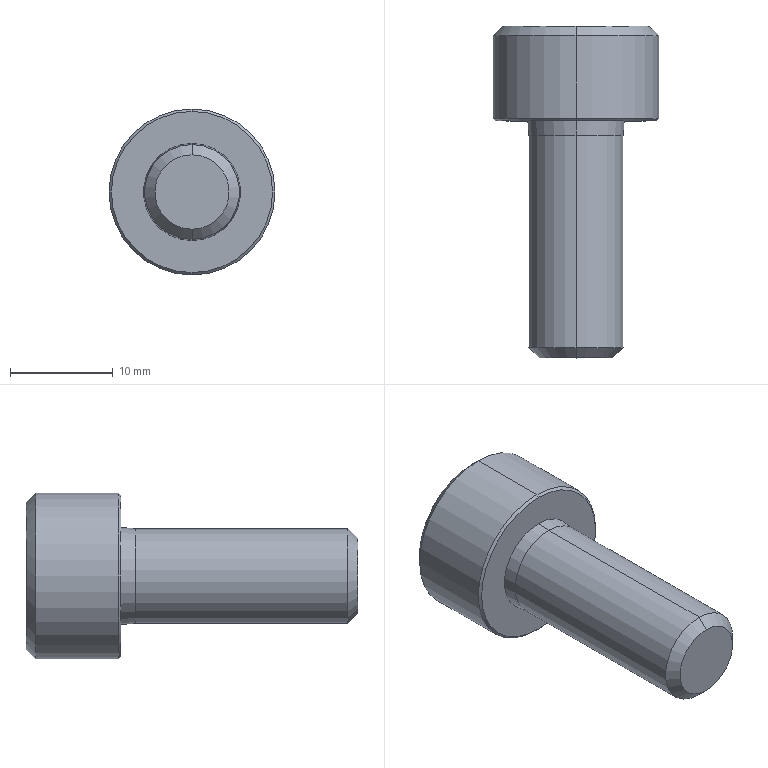Part | SolidWorks | features BaseBody 1 | 1 solid | 36 faces | box 16.154 x 32.308 x 16.154 mm | volume 3185 mm3 | cone 17 | plane 15 | cylinder 4 | commonest cylinder face diameters 9.231 x2 16.154 x2
STEP:
#1=CARTESIAN_POINT('',(207.247,296.414,227.692));
#2=VERTEX_POINT('',#1);
#3=CARTESIAN_POINT('',(207.247,296.414,218.462));
#4=VERTEX_POINT('',#3);
#5=CARTESIAN_POINT('',(207.247,296.414,223.077));
#6=DIRECTION('',(0.,1.,0.));
#7=DIRECTION('',(0.,0.,1.));
#8=AXIS2_PLACEMENT_3D('',#5,#6,#7);
#9=CIRCLE('',#8,4.615);
#10=EDGE_CURVE('',#2,#4,#9,.T.);
#11=ORIENTED_EDGE('',*,*,#10,.T.);
#12=CARTESIAN_POINT('',(207.247,317.115,218.462));
#13=VERTEX_POINT('',#12);
#14=CARTESIAN_POINT('',(207.247,295.423,218.462));
#15=DIRECTION('',(0.,1.,0.));
#16=VECTOR('',#15,1000.);
#17=LINE('',#14,#16);
#18=EDGE_CURVE('',#4,#13,#17,.T.);
#19=ORIENTED_EDGE('',*,*,#18,.T.);
#20=CARTESIAN_POINT('',(207.247,317.115,227.692));
#21=VERTEX_POINT('',#20);
#22=CARTESIAN_POINT('',(207.247,317.115,223.077));
#23=DIRECTION('',(0.,-1.,0.));
#24=DIRECTION('',(0.,0.,1.));
#25=AXIS2_PLACEMENT_3D('',#22,#23,#24);
#26=CIRCLE('',#25,4.615);
#27=EDGE_CURVE('',#13,#21,#26,.T.);
#28=ORIENTED_EDGE('',*,*,#27,.T.);
#29=CARTESIAN_POINT('',(207.247,295.423,227.692));
#30=DIRECTION('',(0.,1.,0.));
#31=VECTOR('',#30,1000.);
#32=LINE('',#29,#31);
#33=EDGE_CURVE('',#2,#21,#32,.T.);
#34=ORIENTED_EDGE('',*,*,#33,.F.);
#35=EDGE_LOOP('',(#11,#19,#28,#34));
#36=FACE_OUTER_BOUND('',#35,.T.);
#37=CARTESIAN_POINT('',(207.247,295.423,223.077));
#38=DIRECTION('',(0.,1.,0.));
#39=DIRECTION('',(0.,0.,1.));
#40=AXIS2_PLACEMENT_3D('',#37,#38,#39);
#41=CYLINDRICAL_SURFACE('',#40,4.615);
#42=ADVANCED_FACE('',(#36),#41,.T.);
#43=CARTESIAN_POINT('',(207.247,295.423,226.701));
#44=VERTEX_POINT('',#43);
#45=CARTESIAN_POINT('',(207.247,295.423,219.453));
#46=VERTEX_POINT('',#45);
#47=CARTESIAN_POINT('',(207.247,295.423,223.077));
#48=DIRECTION('',(0.,1.,0.));
#49=DIRECTION('',(0.,0.,1.));
#50=AXIS2_PLACEMENT_3D('',#47,#48,#49);
#51=CIRCLE('',#50,3.624);
#52=EDGE_CURVE('',#44,#46,#51,.T.);
#53=ORIENTED_EDGE('',*,*,#52,.T.);
#54=CARTESIAN_POINT('',(207.247,296.414,218.462));
#55=DIRECTION('',(0.,0.7071,-0.7071));
#56=VECTOR('',#55,1000.);
#57=LINE('',#54,#56);
#58=EDGE_CURVE('',#46,#4,#57,.T.);
#59=ORIENTED_EDGE('',*,*,#58,.T.);
#60=ORIENTED_EDGE('',*,*,#10,.F.);
#61=CARTESIAN_POINT('',(207.247,296.414,227.692));
#62=DIRECTION('',(0.,0.7071,0.7071));
#63=VECTOR('',#62,1000.);
#64=LINE('',#61,#63);
#65=EDGE_CURVE('',#44,#2,#64,.T.);
#66=ORIENTED_EDGE('',*,*,#65,.F.);
#67=EDGE_LOOP('',(#53,#59,#60,#66));
#68=FACE_OUTER_BOUND('',#67,.T.);
#69=CARTESIAN_POINT('',(207.247,296.414,223.077));
#70=DIRECTION('',(0.,1.,0.));
#71=DIRECTION('',(0.,0.,1.));
#72=AXIS2_PLACEMENT_3D('',#69,#70,#71);
#73=CONICAL_SURFACE('',#72,4.615,0.7854);
#74=ADVANCED_FACE('',(#68),#73,.T.);
#75=ORIENTED_EDGE('',*,*,#27,.F.);
#76=CARTESIAN_POINT('',(207.247,318.5,218.346));
#77=VERTEX_POINT('',#76);
#78=CARTESIAN_POINT('',(207.247,318.5,218.346));
#79=DIRECTION('',(0.,0.9965,-0.08305));
#80=VECTOR('',#79,1000.);
#81=LINE('',#78,#80);
#82=EDGE_CURVE('',#13,#77,#81,.T.);
#83=ORIENTED_EDGE('',*,*,#82,.T.);
#84=CARTESIAN_POINT('',(207.247,318.5,227.808));
#85=VERTEX_POINT('',#84);
#86=CARTESIAN_POINT('',(207.247,318.5,223.077));
#87=DIRECTION('',(0.,-1.,0.));
#88=DIRECTION('',(0.,0.,1.));
#89=AXIS2_PLACEMENT_3D('',#86,#87,#88);
#90=CIRCLE('',#89,4.731);
#91=EDGE_CURVE('',#77,#85,#90,.T.);
#92=ORIENTED_EDGE('',*,*,#91,.T.);
#93=CARTESIAN_POINT('',(207.247,318.5,227.808));
#94=DIRECTION('',(0.,0.9965,0.08305));
#95=VECTOR('',#94,1000.);
#96=LINE('',#93,#95);
#97=EDGE_CURVE('',#21,#85,#96,.T.);
#98=ORIENTED_EDGE('',*,*,#97,.F.);
#99=EDGE_LOOP('',(#75,#83,#92,#98));
#100=FACE_OUTER_BOUND('',#99,.T.);
#101=CARTESIAN_POINT('',(207.247,318.5,223.077));
#102=DIRECTION('',(0.,1.,0.));
#103=DIRECTION('',(0.,0.,1.));
#104=AXIS2_PLACEMENT_3D('',#101,#102,#103);
#105=CONICAL_SURFACE('',#104,4.731,0.08314);
#106=ADVANCED_FACE('',(#100),#105,.T.);
#107=CARTESIAN_POINT('',(207.247,318.5,230.923));
#108=VERTEX_POINT('',#107);
#109=CARTESIAN_POINT('',(207.247,318.5,215.231));
#110=VERTEX_POINT('',#109);
#111=CARTESIAN_POINT('',(207.247,318.5,223.077));
#112=DIRECTION('',(0.,1.,0.));
#113=DIRECTION('',(0.,0.,1.));
#114=AXIS2_PLACEMENT_3D('',#111,#112,#113);
#115=CIRCLE('',#114,7.846);
#116=EDGE_CURVE('',#108,#110,#115,.T.);
#117=ORIENTED_EDGE('',*,*,#116,.T.);
#118=CARTESIAN_POINT('',(207.247,318.731,215.));
#119=VERTEX_POINT('',#118);
#120=CARTESIAN_POINT('',(207.247,318.731,215.));
#121=DIRECTION('',(0.,0.7071,-0.7071));
#122=VECTOR('',#121,1000.);
#123=LINE('',#120,#122);
#124=EDGE_CURVE('',#110,#119,#123,.T.);
#125=ORIENTED_EDGE('',*,*,#124,.T.);
#126=CARTESIAN_POINT('',(207.247,318.731,231.154));
#127=VERTEX_POINT('',#126);
#128=CARTESIAN_POINT('',(207.247,318.731,223.077));
#129=DIRECTION('',(0.,-1.,0.));
#130=DIRECTION('',(0.,0.,-1.));
#131=AXIS2_PLACEMENT_3D('',#128,#129,#130);
#132=CIRCLE('',#131,8.077);
#133=EDGE_CURVE('',#119,#127,#132,.T.);
#134=ORIENTED_EDGE('',*,*,#133,.T.);
#135=CARTESIAN_POINT('',(207.247,318.731,231.154));
#136=DIRECTION('',(0.,0.7071,0.7071));
#137=VECTOR('',#136,1000.);
#138=LINE('',#135,#137);
#139=EDGE_CURVE('',#108,#127,#138,.T.);
#140=ORIENTED_EDGE('',*,*,#139,.F.);
#141=EDGE_LOOP('',(#117,#125,#134,#140));
#142=FACE_OUTER_BOUND('',#141,.T.);
#143=CARTESIAN_POINT('',(207.247,318.731,223.077));
#144=DIRECTION('',(0.,1.,0.));
#145=DIRECTION('',(0.,0.,1.));
#146=AXIS2_PLACEMENT_3D('',#143,#144,#145);
#147=CONICAL_SURFACE('',#146,8.077,0.7854);
#148=ADVANCED_FACE('',(#142),#147,.T.);
#149=ORIENTED_EDGE('',*,*,#133,.F.);
#150=CARTESIAN_POINT('',(207.247,326.808,215.));
#151=VERTEX_POINT('',#150);
#152=CARTESIAN_POINT('',(207.247,295.423,215.));
#153=DIRECTION('',(0.,1.,0.));
#154=VECTOR('',#153,1000.);
#155=LINE('',#152,#154);
#156=EDGE_CURVE('',#119,#151,#155,.T.);
#157=ORIENTED_EDGE('',*,*,#156,.T.);
#158=CARTESIAN_POINT('',(207.247,326.808,231.154));
#159=VERTEX_POINT('',#158);
#160=CARTESIAN_POINT('',(207.247,326.808,223.077));
#161=DIRECTION('',(0.,-1.,0.));
#162=DIRECTION('',(0.,0.,1.));
#163=AXIS2_PLACEMENT_3D('',#160,#161,#162);
#164=CIRCLE('',#163,8.077);
#165=EDGE_CURVE('',#151,#159,#164,.T.);
#166=ORIENTED_EDGE('',*,*,#165,.T.);
#167=CARTESIAN_POINT('',(207.247,295.423,231.154));
#168=DIRECTION('',(0.,1.,0.));
#169=VECTOR('',#168,1000.);
#170=LINE('',#167,#169);
#171=EDGE_CURVE('',#127,#159,#170,.T.);
#172=ORIENTED_EDGE('',*,*,#171,.F.);
#173=EDGE_LOOP('',(#149,#157,#166,#172));
#174=FACE_OUTER_BOUND('',#173,.T.);
#175=CARTESIAN_POINT('',(207.247,295.423,223.077));
#176=DIRECTION('',(0.,1.,0.));
#177=DIRECTION('',(0.,0.,1.));
#178=AXIS2_PLACEMENT_3D('',#175,#176,#177);
#179=CYLINDRICAL_SURFACE('',#178,8.077);
#180=ADVANCED_FACE('',(#174),#179,.T.);
#181=CARTESIAN_POINT('',(207.247,327.731,215.923));
#182=VERTEX_POINT('',#181);
#183=CARTESIAN_POINT('',(207.247,327.731,230.231));
#184=VERTEX_POINT('',#183);
#185=CARTESIAN_POINT('',(207.247,327.731,223.077));
#186=DIRECTION('',(0.,-1.,0.));
#187=DIRECTION('',(0.,0.,-1.));
#188=AXIS2_PLACEMENT_3D('',#185,#186,#187);
#189=CIRCLE('',#188,7.154);
#190=EDGE_CURVE('',#182,#184,#189,.T.);
#191=ORIENTED_EDGE('',*,*,#190,.T.);
#192=CARTESIAN_POINT('',(207.247,326.808,231.154));
#193=DIRECTION('',(0.,-0.7071,0.7071));
#194=VECTOR('',#193,1000.);
#195=LINE('',#192,#194);
#196=EDGE_CURVE('',#184,#159,#195,.T.);
#197=ORIENTED_EDGE('',*,*,#196,.T.);
#198=ORIENTED_EDGE('',*,*,#165,.F.);
#199=CARTESIAN_POINT('',(207.247,326.808,215.));
#200=DIRECTION('',(0.,-0.7071,-0.7071));
#201=VECTOR('',#200,1000.);
#202=LINE('',#199,#201);
#203=EDGE_CURVE('',#182,#151,#202,.T.);
#204=ORIENTED_EDGE('',*,*,#203,.F.);
#205=EDGE_LOOP('',(#191,#197,#198,#204));
#206=FACE_OUTER_BOUND('',#205,.T.);
#207=CARTESIAN_POINT('',(207.247,326.808,223.077));
#208=DIRECTION('',(0.,-1.,0.));
#209=DIRECTION('',(0.,0.,-1.));
#210=AXIS2_PLACEMENT_3D('',#207,#208,#209);
#211=CONICAL_SURFACE('',#210,8.077,0.7854);
#212=ADVANCED_FACE('',(#206),#211,.T.);
#213=CARTESIAN_POINT('',(207.247,327.195,226.538));
#214=VERTEX_POINT('',#213);
#215=CARTESIAN_POINT('',(209.245,327.731,226.538));
#216=VERTEX_POINT('',#215);
#217=CARTESIAN_POINT('',(207.247,327.195,226.538));
#218=CARTESIAN_POINT('',(207.594,327.195,226.538));
#219=CARTESIAN_POINT('',(207.936,327.248,226.538));
#220=CARTESIAN_POINT('',(208.61,327.44,226.538));
#221=CARTESIAN_POINT('',(208.932,327.574,226.538));
#222=CARTESIAN_POINT('',(209.245,327.731,226.538));
#223=B_SPLINE_CURVE_WITH_KNOTS('',3,(#217,#218,#219,#220,#221,#222),.UNSPECIFIED.,.F.,.F.,(4,2,4),(0.002072,0.0031,0.004129),.UNSPECIFIED.);
#224=EDGE_CURVE('',#214,#216,#223,.T.);
#225=ORIENTED_EDGE('',*,*,#224,.F.);
#226=CARTESIAN_POINT('',(207.247,327.731,227.074));
#227=VERTEX_POINT('',#226);
#228=CARTESIAN_POINT('',(207.247,327.731,227.074));
#229=DIRECTION('',(0.,0.7071,0.7071));
#230=VECTOR('',#229,1000.);
#231=LINE('',#228,#230);
#232=EDGE_CURVE('',#214,#227,#231,.T.);
#233=ORIENTED_EDGE('',*,*,#232,.T.);
#234=CARTESIAN_POINT('',(207.247,327.731,223.077));
#235=DIRECTION('',(0.,1.,0.));
#236=DIRECTION('',(0.,0.,1.));
#237=AXIS2_PLACEMENT_3D('',#234,#235,#236);
#238=CIRCLE('',#237,3.997);
#239=EDGE_CURVE('',#227,#216,#238,.T.);
#240=ORIENTED_EDGE('',*,*,#239,.T.);
#241=EDGE_LOOP('',(#225,#233,#240));
#242=FACE_OUTER_BOUND('',#241,.T.);
#243=CARTESIAN_POINT('',(207.247,327.731,223.077));
#244=DIRECTION('',(0.,1.,0.));
#245=DIRECTION('',(0.,0.,1.));
#246=AXIS2_PLACEMENT_3D('',#243,#244,#245);
#247=CONICAL_SURFACE('',#246,3.997,0.7854);
#248=ADVANCED_FACE('',(#242),#247,.F.);
#249=CARTESIAN_POINT('',(207.247,321.117,223.077));
#250=VERTEX_POINT('',#249);
#251=CARTESIAN_POINT('',(207.247,323.115,226.538));
#252=VERTEX_POINT('',#251);
#253=CARTESIAN_POINT('',(207.247,323.115,226.538));
#254=DIRECTION('',(0.,0.5,0.866));
#255=VECTOR('',#254,1000.);
#256=LINE('',#253,#255);
#257=EDGE_CURVE('',#250,#252,#256,.T.);
#258=ORIENTED_EDGE('',*,*,#257,.F.);
#259=CARTESIAN_POINT('',(207.247,323.115,219.615));
#260=VERTEX_POINT('',#259);
#261=CARTESIAN_POINT('',(207.247,323.115,219.615));
#262=DIRECTION('',(0.,0.5,-0.866));
#263=VECTOR('',#262,1000.);
#264=LINE('',#261,#263);
#265=EDGE_CURVE('',#250,#260,#264,.T.);
#266=ORIENTED_EDGE('',*,*,#265,.T.);
#267=CARTESIAN_POINT('',(204.249,323.115,221.346));
#268=VERTEX_POINT('',#267);
#269=CARTESIAN_POINT('',(207.247,323.115,223.077));
#270=DIRECTION('',(0.,-1.,0.));
#271=DIRECTION('',(0.,0.,1.));
#272=AXIS2_PLACEMENT_3D('',#269,#270,#271);
#273=CIRCLE('',#272,3.462);
#274=EDGE_CURVE('',#268,#260,#273,.T.);
#275=ORIENTED_EDGE('',*,*,#274,.F.);
#276=CARTESIAN_POINT('',(204.249,323.115,224.808));
#277=VERTEX_POINT('',#276);
#278=CARTESIAN_POINT('',(207.247,323.115,223.077));
#279=DIRECTION('',(0.,-1.,0.));
#280=DIRECTION('',(0.,0.,1.));
#281=AXIS2_PLACEMENT_3D('',#278,#279,#280);
#282=CIRCLE('',#281,3.462);
#283=EDGE_CURVE('',#277,#268,#282,.T.);
#284=ORIENTED_EDGE('',*,*,#283,.F.);
#285=CARTESIAN_POINT('',(207.247,323.115,223.077));
#286=DIRECTION('',(0.,-1.,0.));
#287=DIRECTION('',(0.,0.,1.));
#288=AXIS2_PLACEMENT_3D('',#285,#286,#287);
#289=CIRCLE('',#288,3.462);
#290=EDGE_CURVE('',#252,#277,#289,.T.);
#291=ORIENTED_EDGE('',*,*,#290,.F.);
#292=EDGE_LOOP('',(#258,#266,#275,#284,#291));
#293=FACE_OUTER_BOUND('',#292,.T.);
#294=CARTESIAN_POINT('',(207.247,323.115,223.077));
#295=DIRECTION('',(0.,1.,0.));
#296=DIRECTION('',(0.,0.,1.));
#297=AXIS2_PLACEMENT_3D('',#294,#295,#296);
#298=CONICAL_SURFACE('',#297,3.462,1.047);
#299=ADVANCED_FACE('',(#293),#298,.F.);
#300=ORIENTED_EDGE('',*,*,#18,.F.);
#301=CARTESIAN_POINT('',(207.247,296.414,223.077));
#302=DIRECTION('',(0.,1.,0.));
#303=DIRECTION('',(0.,0.,1.));
#304=AXIS2_PLACEMENT_3D('',#301,#302,#303);
#305=CIRCLE('',#304,4.615);
#306=EDGE_CURVE('',#4,#2,#305,.T.);
#307=ORIENTED_EDGE('',*,*,#306,.T.);
#308=ORIENTED_EDGE('',*,*,#33,.T.);
#309=CARTESIAN_POINT('',(207.247,317.115,223.077));
#310=DIRECTION('',(0.,-1.,0.));
#311=DIRECTION('',(0.,0.,1.));
#312=AXIS2_PLACEMENT_3D('',#309,#310,#311);
#313=CIRCLE('',#312,4.615);
#314=EDGE_CURVE('',#21,#13,#313,.T.);
#315=ORIENTED_EDGE('',*,*,#314,.T.);
#316=EDGE_LOOP('',(#300,#307,#308,#315));
#317=FACE_OUTER_BOUND('',#316,.T.);
#318=CARTESIAN_POINT('',(207.247,295.423,223.077));
#319=DIRECTION('',(0.,1.,0.));
#320=DIRECTION('',(0.,0.,1.));
#321=AXIS2_PLACEMENT_3D('',#318,#319,#320);
#322=CYLINDRICAL_SURFACE('',#321,4.615);
#323=ADVANCED_FACE('',(#317),#322,.T.);
#324=ORIENTED_EDGE('',*,*,#58,.F.);
#325=CARTESIAN_POINT('',(207.247,295.423,223.077));
#326=DIRECTION('',(0.,1.,0.));
#327=DIRECTION('',(0.,0.,1.));
#328=AXIS2_PLACEMENT_3D('',#325,#326,#327);
#329=CIRCLE('',#328,3.624);
#330=EDGE_CURVE('',#46,#44,#329,.T.);
#331=ORIENTED_EDGE('',*,*,#330,.T.);
#332=ORIENTED_EDGE('',*,*,#65,.T.);
#333=ORIENTED_EDGE('',*,*,#306,.F.);
#334=EDGE_LOOP('',(#324,#331,#332,#333));
#335=FACE_OUTER_BOUND('',#334,.T.);
#336=CARTESIAN_POINT('',(207.247,296.414,223.077));
#337=DIRECTION('',(0.,1.,0.));
#338=DIRECTION('',(0.,0.,1.));
#339=AXIS2_PLACEMENT_3D('',#336,#337,#338);
#340=CONICAL_SURFACE('',#339,4.615,0.7854);
#341=ADVANCED_FACE('',(#335),#340,.T.);
#342=ORIENTED_EDGE('',*,*,#82,.F.);
#343=ORIENTED_EDGE('',*,*,#314,.F.);
#344=ORIENTED_EDGE('',*,*,#97,.T.);
#345=CARTESIAN_POINT('',(207.247,318.5,223.077));
#346=DIRECTION('',(0.,-1.,0.));
#347=DIRECTION('',(0.,0.,1.));
#348=AXIS2_PLACEMENT_3D('',#345,#346,#347);
#349=CIRCLE('',#348,4.731);
#350=EDGE_CURVE('',#85,#77,#349,.T.);
#351=ORIENTED_EDGE('',*,*,#350,.T.);
#352=EDGE_LOOP('',(#342,#343,#344,#351));
#353=FACE_OUTER_BOUND('',#352,.T.);
#354=CARTESIAN_POINT('',(207.247,318.5,223.077));
#355=DIRECTION('',(0.,1.,0.));
#356=DIRECTION('',(0.,0.,1.));
#357=AXIS2_PLACEMENT_3D('',#354,#355,#356);
#358=CONICAL_SURFACE('',#357,4.731,0.08314);
#359=ADVANCED_FACE('',(#353),#358,.T.);
#360=ORIENTED_EDGE('',*,*,#52,.F.);
#361=ORIENTED_EDGE('',*,*,#330,.F.);
#362=EDGE_LOOP('',(#360,#361));
#363=FACE_OUTER_BOUND('',#362,.T.);
#364=CARTESIAN_POINT('',(207.247,295.423,219.453));
#365=DIRECTION('',(0.,1.,0.));
#366=DIRECTION('',(0.,0.,1.));
#367=AXIS2_PLACEMENT_3D('',#364,#365,#366);
#368=PLANE('',#367);
#369=ADVANCED_FACE('',(#363),#368,.F.);
#370=ORIENTED_EDGE('',*,*,#350,.F.);
#371=ORIENTED_EDGE('',*,*,#91,.F.);
#372=EDGE_LOOP('',(#370,#371));
#373=FACE_BOUND('',#372,.T.);
#374=ORIENTED_EDGE('',*,*,#116,.F.);
#375=CARTESIAN_POINT('',(207.247,318.5,223.077));
#376=DIRECTION('',(0.,1.,0.));
#377=DIRECTION('',(0.,0.,1.));
#378=AXIS2_PLACEMENT_3D('',#375,#376,#377);
#379=CIRCLE('',#378,7.846);
#380=EDGE_CURVE('',#110,#108,#379,.T.);
#381=ORIENTED_EDGE('',*,*,#380,.F.);
#382=EDGE_LOOP('',(#374,#381));
#383=FACE_OUTER_BOUND('',#382,.T.);
#384=CARTESIAN_POINT('',(207.247,318.5,215.231));
#385=DIRECTION('',(0.,1.,0.));
#386=DIRECTION('',(0.,0.,1.));
#387=AXIS2_PLACEMENT_3D('',#384,#385,#386);
#388=PLANE('',#387);
#389=ADVANCED_FACE('',(#373,#383),#388,.F.);
#390=ORIENTED_EDGE('',*,*,#124,.F.);
#391=ORIENTED_EDGE('',*,*,#380,.T.);
#392=ORIENTED_EDGE('',*,*,#139,.T.);
#393=CARTESIAN_POINT('',(207.247,318.731,223.077));
#394=DIRECTION('',(0.,-1.,0.));
#395=DIRECTION('',(0.,0.,-1.));
#396=AXIS2_PLACEMENT_3D('',#393,#394,#395);
#397=CIRCLE('',#396,8.077);
#398=EDGE_CURVE('',#127,#119,#397,.T.);
#399=ORIENTED_EDGE('',*,*,#398,.T.);
#400=EDGE_LOOP('',(#390,#391,#392,#399));
#401=FACE_OUTER_BOUND('',#400,.T.);
#402=CARTESIAN_POINT('',(207.247,318.731,223.077));
#403=DIRECTION('',(0.,1.,0.));
#404=DIRECTION('',(0.,0.,1.));
#405=AXIS2_PLACEMENT_3D('',#402,#403,#404);
#406=CONICAL_SURFACE('',#405,8.077,0.7854);
#407=ADVANCED_FACE('',(#401),#406,.T.);
#408=ORIENTED_EDGE('',*,*,#156,.F.);
#409=ORIENTED_EDGE('',*,*,#398,.F.);
#410=ORIENTED_EDGE('',*,*,#171,.T.);
#411=CARTESIAN_POINT('',(207.247,326.808,223.077));
#412=DIRECTION('',(0.,-1.,0.));
#413=DIRECTION('',(0.,0.,1.));
#414=AXIS2_PLACEMENT_3D('',#411,#412,#413);
#415=CIRCLE('',#414,8.077);
#416=EDGE_CURVE('',#159,#151,#415,.T.);
#417=ORIENTED_EDGE('',*,*,#416,.T.);
#418=EDGE_LOOP('',(#408,#409,#410,#417));
#419=FACE_OUTER_BOUND('',#418,.T.);
#420=CARTESIAN_POINT('',(207.247,295.423,223.077));
#421=DIRECTION('',(0.,1.,0.));
#422=DIRECTION('',(0.,0.,1.));
#423=AXIS2_PLACEMENT_3D('',#420,#421,#422);
#424=CYLINDRICAL_SURFACE('',#423,8.077);
#425=ADVANCED_FACE('',(#419),#424,.T.);
#426=ORIENTED_EDGE('',*,*,#196,.F.);
#427=CARTESIAN_POINT('',(207.247,327.731,223.077));
#428=DIRECTION('',(0.,-1.,0.));
#429=DIRECTION('',(0.,0.,-1.));
#430=AXIS2_PLACEMENT_3D('',#427,#428,#429);
#431=CIRCLE('',#430,7.154);
#432=EDGE_CURVE('',#184,#182,#431,.T.);
#433=ORIENTED_EDGE('',*,*,#432,.T.);
#434=ORIENTED_EDGE('',*,*,#203,.T.);
#435=ORIENTED_EDGE('',*,*,#416,.F.);
#436=EDGE_LOOP('',(#426,#433,#434,#435));
#437=FACE_OUTER_BOUND('',#436,.T.);
#438=CARTESIAN_POINT('',(207.247,326.808,223.077));
#439=DIRECTION('',(0.,-1.,0.));
#440=DIRECTION('',(0.,0.,-1.));
#441=AXIS2_PLACEMENT_3D('',#438,#439,#440);
#442=CONICAL_SURFACE('',#441,8.077,0.7854);
#443=ADVANCED_FACE('',(#437),#442,.T.);
#444=CARTESIAN_POINT('',(211.244,327.731,223.077));
#445=VERTEX_POINT('',#444);
#446=CARTESIAN_POINT('',(207.247,327.731,223.077));
#447=DIRECTION('',(0.,1.,0.));
#448=DIRECTION('',(0.,0.,1.));
#449=AXIS2_PLACEMENT_3D('',#446,#447,#448);
#450=CIRCLE('',#449,3.997);
#451=EDGE_CURVE('',#216,#445,#450,.T.);
#452=ORIENTED_EDGE('',*,*,#451,.F.);
#453=ORIENTED_EDGE('',*,*,#239,.F.);
#454=CARTESIAN_POINT('',(205.248,327.731,226.538));
#455=VERTEX_POINT('',#454);
#456=CARTESIAN_POINT('',(207.247,327.731,223.077));
#457=DIRECTION('',(0.,1.,0.));
#458=DIRECTION('',(0.,0.,1.));
#459=AXIS2_PLACEMENT_3D('',#456,#457,#458);
#460=CIRCLE('',#459,3.997);
#461=EDGE_CURVE('',#455,#227,#460,.T.);
#462=ORIENTED_EDGE('',*,*,#461,.F.);
#463=CARTESIAN_POINT('',(203.249,327.731,223.077));
#464=VERTEX_POINT('',#463);
#465=CARTESIAN_POINT('',(207.247,327.731,223.077));
#466=DIRECTION('',(0.,1.,0.));
#467=DIRECTION('',(0.,0.,1.));
#468=AXIS2_PLACEMENT_3D('',#465,#466,#467);
#469=CIRCLE('',#468,3.997);
#470=EDGE_CURVE('',#464,#455,#469,.T.);
#471=ORIENTED_EDGE('',*,*,#470,.F.);
#472=CARTESIAN_POINT('',(205.248,327.731,219.615));
#473=VERTEX_POINT('',#472);
#474=CARTESIAN_POINT('',(207.247,327.731,223.077));
#475=DIRECTION('',(0.,1.,0.));
#476=DIRECTION('',(0.,0.,1.));
#477=AXIS2_PLACEMENT_3D('',#474,#475,#476);
#478=CIRCLE('',#477,3.997);
#479=EDGE_CURVE('',#473,#464,#478,.T.);
#480=ORIENTED_EDGE('',*,*,#479,.F.);
#481=CARTESIAN_POINT('',(209.245,327.731,219.615));
#482=VERTEX_POINT('',#481);
#483=CARTESIAN_POINT('',(207.247,327.731,223.077));
#484=DIRECTION('',(0.,1.,0.));
#485=DIRECTION('',(0.,0.,1.));
#486=AXIS2_PLACEMENT_3D('',#483,#484,#485);
#487=CIRCLE('',#486,3.997);
#488=EDGE_CURVE('',#482,#473,#487,.T.);
#489=ORIENTED_EDGE('',*,*,#488,.F.);
#490=CARTESIAN_POINT('',(207.247,327.731,223.077));
#491=DIRECTION('',(0.,1.,0.));
#492=DIRECTION('',(0.,0.,1.));
#493=AXIS2_PLACEMENT_3D('',#490,#491,#492);
#494=CIRCLE('',#493,3.997);
#495=EDGE_CURVE('',#445,#482,#494,.T.);
#496=ORIENTED_EDGE('',*,*,#495,.F.);
#497=EDGE_LOOP('',(#452,#453,#462,#471,#480,#489,#496));
#498=FACE_BOUND('',#497,.T.);
#499=ORIENTED_EDGE('',*,*,#190,.F.);
#500=ORIENTED_EDGE('',*,*,#432,.F.);
#501=EDGE_LOOP('',(#499,#500));
#502=FACE_OUTER_BOUND('',#501,.T.);
#503=CARTESIAN_POINT('',(207.247,327.731,219.08));
#504=DIRECTION('',(0.,-1.,0.));
#505=DIRECTION('',(0.,0.,-1.));
#506=AXIS2_PLACEMENT_3D('',#503,#504,#505);
#507=PLANE('',#506);
#508=ADVANCED_FACE('',(#498,#502),#507,.F.);
#509=CARTESIAN_POINT('',(211.244,327.731,223.077));
#510=CARTESIAN_POINT('',(211.087,327.575,222.806));
#511=CARTESIAN_POINT('',(210.928,327.442,222.53));
#512=CARTESIAN_POINT('',(210.68,327.3,222.1));
#513=CARTESIAN_POINT('',(210.596,327.262,221.955));
#514=CARTESIAN_POINT('',(210.424,327.21,221.657));
#515=CARTESIAN_POINT('',(210.335,327.196,221.504));
#516=CARTESIAN_POINT('',(210.074,327.195,221.05));
#517=CARTESIAN_POINT('',(209.902,327.247,220.753));
#518=CARTESIAN_POINT('',(209.564,327.439,220.168));
#519=CARTESIAN_POINT('',(209.402,327.574,219.887));
#520=CARTESIAN_POINT('',(209.245,327.731,219.615));
#521=B_SPLINE_CURVE_WITH_KNOTS('',3,(#509,#510,#511,#512,#513,#514,#515,#516,#517,#518,#519,#520),.UNSPECIFIED.,.F.,.F.,(4,2,2,2,2,4),(0.,0.001032,0.001548,0.002064,0.003097,0.004129),.UNSPECIFIED.);
#522=EDGE_CURVE('',#445,#482,#521,.T.);
#523=ORIENTED_EDGE('',*,*,#522,.F.);
#524=ORIENTED_EDGE('',*,*,#495,.T.);
#525=EDGE_LOOP('',(#523,#524));
#526=FACE_OUTER_BOUND('',#525,.T.);
#527=CARTESIAN_POINT('',(207.247,327.731,223.077));
#528=DIRECTION('',(0.,1.,0.));
#529=DIRECTION('',(0.,0.,1.));
#530=AXIS2_PLACEMENT_3D('',#527,#528,#529);
#531=CONICAL_SURFACE('',#530,3.997,0.7854);
#532=ADVANCED_FACE('',(#526),#531,.F.);
#533=CARTESIAN_POINT('',(209.245,327.731,226.538));
#534=CARTESIAN_POINT('',(209.401,327.575,226.268));
#535=CARTESIAN_POINT('',(209.561,327.442,225.991));
#536=CARTESIAN_POINT('',(209.809,327.3,225.562));
#537=CARTESIAN_POINT('',(209.893,327.262,225.416));
#538=CARTESIAN_POINT('',(210.065,327.21,225.118));
#539=CARTESIAN_POINT('',(210.153,327.196,224.965));
#540=CARTESIAN_POINT('',(210.415,327.195,224.512));
#541=CARTESIAN_POINT('',(210.587,327.247,224.215));
#542=CARTESIAN_POINT('',(210.925,327.439,223.629));
#543=CARTESIAN_POINT('',(211.087,327.574,223.349));
#544=CARTESIAN_POINT('',(211.244,327.731,223.077));
#545=B_SPLINE_CURVE_WITH_KNOTS('',3,(#533,#534,#535,#536,#537,#538,#539,#540,#541,#542,#543,#544),.UNSPECIFIED.,.F.,.F.,(4,2,2,2,2,4),(0.,0.001032,0.001548,0.002064,0.003097,0.004129),.UNSPECIFIED.);
#546=EDGE_CURVE('',#216,#445,#545,.T.);
#547=ORIENTED_EDGE('',*,*,#546,.F.);
#548=ORIENTED_EDGE('',*,*,#451,.T.);
#549=EDGE_LOOP('',(#547,#548));
#550=FACE_OUTER_BOUND('',#549,.T.);
#551=CARTESIAN_POINT('',(207.247,327.731,223.077));
#552=DIRECTION('',(0.,1.,0.));
#553=DIRECTION('',(0.,0.,1.));
#554=AXIS2_PLACEMENT_3D('',#551,#552,#553);
#555=CONICAL_SURFACE('',#554,3.997,0.7854);
#556=ADVANCED_FACE('',(#550),#555,.F.);
#557=ORIENTED_EDGE('',*,*,#232,.F.);
#558=CARTESIAN_POINT('',(205.248,327.731,226.538));
#559=CARTESIAN_POINT('',(205.561,327.574,226.538));
#560=CARTESIAN_POINT('',(205.882,327.441,226.538));
#561=CARTESIAN_POINT('',(206.38,327.299,226.538));
#562=CARTESIAN_POINT('',(206.549,327.261,226.538));
#563=CARTESIAN_POINT('',(206.894,327.209,226.538));
#564=CARTESIAN_POINT('',(207.071,327.195,226.538));
#565=CARTESIAN_POINT('',(207.247,327.195,226.538));
#566=B_SPLINE_CURVE_WITH_KNOTS('',3,(#558,#559,#560,#561,#562,#563,#564,#565),.UNSPECIFIED.,.F.,.F.,(4,2,2,4),(0.,0.001036,0.001554,0.002072),.UNSPECIFIED.);
#567=EDGE_CURVE('',#455,#214,#566,.T.);
#568=ORIENTED_EDGE('',*,*,#567,.F.);
#569=ORIENTED_EDGE('',*,*,#461,.T.);
#570=EDGE_LOOP('',(#557,#568,#569));
#571=FACE_OUTER_BOUND('',#570,.T.);
#572=CARTESIAN_POINT('',(207.247,327.731,223.077));
#573=DIRECTION('',(0.,1.,0.));
#574=DIRECTION('',(0.,0.,1.));
#575=AXIS2_PLACEMENT_3D('',#572,#573,#574);
#576=CONICAL_SURFACE('',#575,3.997,0.7854);
#577=ADVANCED_FACE('',(#571),#576,.F.);
#578=CARTESIAN_POINT('',(203.249,327.731,223.077));
#579=CARTESIAN_POINT('',(203.406,327.575,223.347));
#580=CARTESIAN_POINT('',(203.565,327.442,223.624));
#581=CARTESIAN_POINT('',(203.813,327.3,224.054));
#582=CARTESIAN_POINT('',(203.898,327.262,224.199));
#583=CARTESIAN_POINT('',(204.069,327.21,224.497));
#584=CARTESIAN_POINT('',(204.158,327.196,224.65));
#585=CARTESIAN_POINT('',(204.42,327.195,225.104));
#586=CARTESIAN_POINT('',(204.591,327.247,225.401));
#587=CARTESIAN_POINT('',(204.929,327.439,225.986));
#588=CARTESIAN_POINT('',(205.091,327.574,226.266));
#589=CARTESIAN_POINT('',(205.248,327.731,226.538));
#590=B_SPLINE_CURVE_WITH_KNOTS('',3,(#578,#579,#580,#581,#582,#583,#584,#585,#586,#587,#588,#589),.UNSPECIFIED.,.F.,.F.,(4,2,2,2,2,4),(0.,0.001032,0.001548,0.002064,0.003097,0.004129),.UNSPECIFIED.);
#591=EDGE_CURVE('',#464,#455,#590,.T.);
#592=ORIENTED_EDGE('',*,*,#591,.F.);
#593=ORIENTED_EDGE('',*,*,#470,.T.);
#594=EDGE_LOOP('',(#592,#593));
#595=FACE_OUTER_BOUND('',#594,.T.);
#596=CARTESIAN_POINT('',(207.247,327.731,223.077));
#597=DIRECTION('',(0.,1.,0.));
#598=DIRECTION('',(0.,0.,1.));
#599=AXIS2_PLACEMENT_3D('',#596,#597,#598);
#600=CONICAL_SURFACE('',#599,3.997,0.7854);
#601=ADVANCED_FACE('',(#595),#600,.F.);
#602=CARTESIAN_POINT('',(205.248,327.731,219.615));
#603=CARTESIAN_POINT('',(205.092,327.575,219.886));
#604=CARTESIAN_POINT('',(204.932,327.442,220.162));
#605=CARTESIAN_POINT('',(204.684,327.3,220.592));
#606=CARTESIAN_POINT('',(204.6,327.262,220.738));
#607=CARTESIAN_POINT('',(204.428,327.21,221.035));
#608=CARTESIAN_POINT('',(204.34,327.196,221.189));
#609=CARTESIAN_POINT('',(204.078,327.195,221.642));
#610=CARTESIAN_POINT('',(203.906,327.247,221.939));
#611=CARTESIAN_POINT('',(203.568,327.439,222.525));
#612=CARTESIAN_POINT('',(203.407,327.574,222.805));
#613=CARTESIAN_POINT('',(203.249,327.731,223.077));
#614=B_SPLINE_CURVE_WITH_KNOTS('',3,(#602,#603,#604,#605,#606,#607,#608,#609,#610,#611,#612,#613),.UNSPECIFIED.,.F.,.F.,(4,2,2,2,2,4),(0.,0.001032,0.001548,0.002064,0.003097,0.004129),.UNSPECIFIED.);
#615=EDGE_CURVE('',#473,#464,#614,.T.);
#616=ORIENTED_EDGE('',*,*,#615,.F.);
#617=ORIENTED_EDGE('',*,*,#479,.T.);
#618=EDGE_LOOP('',(#616,#617));
#619=FACE_OUTER_BOUND('',#618,.T.);
#620=CARTESIAN_POINT('',(207.247,327.731,223.077));
#621=DIRECTION('',(0.,1.,0.));
#622=DIRECTION('',(0.,0.,1.));
#623=AXIS2_PLACEMENT_3D('',#620,#621,#622);
#624=CONICAL_SURFACE('',#623,3.997,0.7854);
#625=ADVANCED_FACE('',(#619),#624,.F.);
#626=CARTESIAN_POINT('',(209.245,327.731,219.615));
#627=CARTESIAN_POINT('',(208.933,327.575,219.615));
#628=CARTESIAN_POINT('',(208.613,327.442,219.615));
#629=CARTESIAN_POINT('',(208.117,327.3,219.615));
#630=CARTESIAN_POINT('',(207.949,327.262,219.615));
#631=CARTESIAN_POINT('',(207.605,327.21,219.615));
#632=CARTESIAN_POINT('',(207.428,327.196,219.615));
#633=CARTESIAN_POINT('',(206.905,327.195,219.615));
#634=CARTESIAN_POINT('',(206.562,327.247,219.615));
#635=CARTESIAN_POINT('',(205.886,327.439,219.615));
#636=CARTESIAN_POINT('',(205.562,327.574,219.615));
#637=CARTESIAN_POINT('',(205.248,327.731,219.615));
#638=B_SPLINE_CURVE_WITH_KNOTS('',3,(#626,#627,#628,#629,#630,#631,#632,#633,#634,#635,#636,#637),.UNSPECIFIED.,.F.,.F.,(4,2,2,2,2,4),(0.,0.001032,0.001548,0.002064,0.003097,0.004129),.UNSPECIFIED.);
#639=EDGE_CURVE('',#482,#473,#638,.T.);
#640=ORIENTED_EDGE('',*,*,#639,.F.);
#641=ORIENTED_EDGE('',*,*,#488,.T.);
#642=EDGE_LOOP('',(#640,#641));
#643=FACE_OUTER_BOUND('',#642,.T.);
#644=CARTESIAN_POINT('',(207.247,327.731,223.077));
#645=DIRECTION('',(0.,1.,0.));
#646=DIRECTION('',(0.,0.,1.));
#647=AXIS2_PLACEMENT_3D('',#644,#645,#646);
#648=CONICAL_SURFACE('',#647,3.997,0.7854);
#649=ADVANCED_FACE('',(#643),#648,.F.);
#650=CARTESIAN_POINT('',(209.245,323.115,219.615));
#651=VERTEX_POINT('',#650);
#652=CARTESIAN_POINT('',(209.245,323.115,219.615));
#653=DIRECTION('',(0.,1.,0.));
#654=VECTOR('',#653,1000.);
#655=LINE('',#652,#654);
#656=EDGE_CURVE('',#651,#482,#655,.T.);
#657=ORIENTED_EDGE('',*,*,#656,.F.);
#658=CARTESIAN_POINT('',(210.244,323.115,221.346));
#659=VERTEX_POINT('',#658);
#660=CARTESIAN_POINT('',(211.244,323.115,223.077));
#661=DIRECTION('',(-0.5,0.,-0.866));
#662=VECTOR('',#661,1000.);
#663=LINE('',#660,#662);
#664=EDGE_CURVE('',#659,#651,#663,.T.);
#665=ORIENTED_EDGE('',*,*,#664,.F.);
#666=CARTESIAN_POINT('',(211.244,323.115,223.077));
#667=VERTEX_POINT('',#666);
#668=CARTESIAN_POINT('',(211.244,323.115,223.077));
#669=DIRECTION('',(-0.5,0.,-0.866));
#670=VECTOR('',#669,1000.);
#671=LINE('',#668,#670);
#672=EDGE_CURVE('',#667,#659,#671,.T.);
#673=ORIENTED_EDGE('',*,*,#672,.F.);
#674=CARTESIAN_POINT('',(211.244,323.115,223.077));
#675=DIRECTION('',(0.,-1.,0.));
#676=VECTOR('',#675,1000.);
#677=LINE('',#674,#676);
#678=EDGE_CURVE('',#445,#667,#677,.T.);
#679=ORIENTED_EDGE('',*,*,#678,.F.);
#680=ORIENTED_EDGE('',*,*,#522,.T.);
#681=EDGE_LOOP('',(#657,#665,#673,#679,#680));
#682=FACE_OUTER_BOUND('',#681,.T.);
#683=CARTESIAN_POINT('',(211.244,323.115,223.077));
#684=DIRECTION('',(0.866,0.,-0.5));
#685=DIRECTION('',(-0.5,0.,-0.866));
#686=AXIS2_PLACEMENT_3D('',#683,#684,#685);
#687=PLANE('',#686);
#688=ADVANCED_FACE('',(#682),#687,.F.);
#689=ORIENTED_EDGE('',*,*,#678,.T.);
#690=CARTESIAN_POINT('',(210.244,323.115,224.808));
#691=VERTEX_POINT('',#690);
#692=CARTESIAN_POINT('',(209.245,323.115,226.538));
#693=DIRECTION('',(0.5,0.,-0.866));
#694=VECTOR('',#693,1000.);
#695=LINE('',#692,#694);
#696=EDGE_CURVE('',#691,#667,#695,.T.);
#697=ORIENTED_EDGE('',*,*,#696,.F.);
#698=CARTESIAN_POINT('',(209.245,323.115,226.538));
#699=VERTEX_POINT('',#698);
#700=CARTESIAN_POINT('',(209.245,323.115,226.538));
#701=DIRECTION('',(0.5,0.,-0.866));
#702=VECTOR('',#701,1000.);
#703=LINE('',#700,#702);
#704=EDGE_CURVE('',#699,#691,#703,.T.);
#705=ORIENTED_EDGE('',*,*,#704,.F.);
#706=CARTESIAN_POINT('',(209.245,323.115,226.538));
#707=DIRECTION('',(0.,-1.,0.));
#708=VECTOR('',#707,1000.);
#709=LINE('',#706,#708);
#710=EDGE_CURVE('',#216,#699,#709,.T.);
#711=ORIENTED_EDGE('',*,*,#710,.F.);
#712=ORIENTED_EDGE('',*,*,#546,.T.);
#713=EDGE_LOOP('',(#689,#697,#705,#711,#712));
#714=FACE_OUTER_BOUND('',#713,.T.);
#715=CARTESIAN_POINT('',(209.245,323.115,226.538));
#716=DIRECTION('',(0.866,0.,0.5));
#717=DIRECTION('',(0.5,0.,-0.866));
#718=AXIS2_PLACEMENT_3D('',#715,#716,#717);
#719=PLANE('',#718);
#720=ADVANCED_FACE('',(#714),#719,.F.);
#721=ORIENTED_EDGE('',*,*,#710,.T.);
#722=CARTESIAN_POINT('',(205.248,323.115,226.538));
#723=DIRECTION('',(1.,0.,0.));
#724=VECTOR('',#723,1000.);
#725=LINE('',#722,#724);
#726=EDGE_CURVE('',#252,#699,#725,.T.);
#727=ORIENTED_EDGE('',*,*,#726,.F.);
#728=CARTESIAN_POINT('',(205.248,323.115,226.538));
#729=VERTEX_POINT('',#728);
#730=CARTESIAN_POINT('',(205.248,323.115,226.538));
#731=DIRECTION('',(1.,0.,0.));
#732=VECTOR('',#731,1000.);
#733=LINE('',#730,#732);
#734=EDGE_CURVE('',#729,#252,#733,.T.);
#735=ORIENTED_EDGE('',*,*,#734,.F.);
#736=CARTESIAN_POINT('',(205.248,323.115,226.538));
#737=DIRECTION('',(0.,-1.,0.));
#738=VECTOR('',#737,1000.);
#739=LINE('',#736,#738);
#740=EDGE_CURVE('',#455,#729,#739,.T.);
#741=ORIENTED_EDGE('',*,*,#740,.F.);
#742=ORIENTED_EDGE('',*,*,#567,.T.);
#743=ORIENTED_EDGE('',*,*,#224,.T.);
#744=EDGE_LOOP('',(#721,#727,#735,#741,#742,#743));
#745=FACE_OUTER_BOUND('',#744,.T.);
#746=CARTESIAN_POINT('',(205.248,323.115,226.538));
#747=DIRECTION('',(0.,0.,1.));
#748=DIRECTION('',(1.,0.,0.));
#749=AXIS2_PLACEMENT_3D('',#746,#747,#748);
#750=PLANE('',#749);
#751=ADVANCED_FACE('',(#745),#750,.F.);
#752=ORIENTED_EDGE('',*,*,#740,.T.);
#753=CARTESIAN_POINT('',(203.249,323.115,223.077));
#754=DIRECTION('',(0.5,0.,0.866));
#755=VECTOR('',#754,1000.);
#756=LINE('',#753,#755);
#757=EDGE_CURVE('',#277,#729,#756,.T.);
#758=ORIENTED_EDGE('',*,*,#757,.F.);
#759=CARTESIAN_POINT('',(203.249,323.115,223.077));
#760=VERTEX_POINT('',#759);
#761=CARTESIAN_POINT('',(203.249,323.115,223.077));
#762=DIRECTION('',(0.5,0.,0.866));
#763=VECTOR('',#762,1000.);
#764=LINE('',#761,#763);
#765=EDGE_CURVE('',#760,#277,#764,.T.);
#766=ORIENTED_EDGE('',*,*,#765,.F.);
#767=CARTESIAN_POINT('',(203.249,323.115,223.077));
#768=DIRECTION('',(0.,-1.,0.));
#769=VECTOR('',#768,1000.);
#770=LINE('',#767,#769);
#771=EDGE_CURVE('',#464,#760,#770,.T.);
#772=ORIENTED_EDGE('',*,*,#771,.F.);
#773=ORIENTED_EDGE('',*,*,#591,.T.);
#774=EDGE_LOOP('',(#752,#758,#766,#772,#773));
#775=FACE_OUTER_BOUND('',#774,.T.);
#776=CARTESIAN_POINT('',(203.249,323.115,223.077));
#777=DIRECTION('',(-0.866,0.,0.5));
#778=DIRECTION('',(0.5,0.,0.866));
#779=AXIS2_PLACEMENT_3D('',#776,#777,#778);
#780=PLANE('',#779);
#781=ADVANCED_FACE('',(#775),#780,.F.);
#782=ORIENTED_EDGE('',*,*,#771,.T.);
#783=CARTESIAN_POINT('',(205.248,323.115,219.615));
#784=DIRECTION('',(-0.5,0.,0.866));
#785=VECTOR('',#784,1000.);
#786=LINE('',#783,#785);
#787=EDGE_CURVE('',#268,#760,#786,.T.);
#788=ORIENTED_EDGE('',*,*,#787,.F.);
#789=CARTESIAN_POINT('',(205.248,323.115,219.615));
#790=VERTEX_POINT('',#789);
#791=CARTESIAN_POINT('',(205.248,323.115,219.615));
#792=DIRECTION('',(-0.5,0.,0.866));
#793=VECTOR('',#792,1000.);
#794=LINE('',#791,#793);
#795=EDGE_CURVE('',#790,#268,#794,.T.);
#796=ORIENTED_EDGE('',*,*,#795,.F.);
#797=CARTESIAN_POINT('',(205.248,323.115,219.615));
#798=DIRECTION('',(0.,-1.,0.));
#799=VECTOR('',#798,1000.);
#800=LINE('',#797,#799);
#801=EDGE_CURVE('',#473,#790,#800,.T.);
#802=ORIENTED_EDGE('',*,*,#801,.F.);
#803=ORIENTED_EDGE('',*,*,#615,.T.);
#804=EDGE_LOOP('',(#782,#788,#796,#802,#803));
#805=FACE_OUTER_BOUND('',#804,.T.);
#806=CARTESIAN_POINT('',(205.248,323.115,219.615));
#807=DIRECTION('',(-0.866,0.,-0.5));
#808=DIRECTION('',(-0.5,0.,0.866));
#809=AXIS2_PLACEMENT_3D('',#806,#807,#808);
#810=PLANE('',#809);
#811=ADVANCED_FACE('',(#805),#810,.F.);
#812=ORIENTED_EDGE('',*,*,#801,.T.);
#813=CARTESIAN_POINT('',(209.245,323.115,219.615));
#814=DIRECTION('',(-1.,0.,0.));
#815=VECTOR('',#814,1000.);
#816=LINE('',#813,#815);
#817=EDGE_CURVE('',#260,#790,#816,.T.);
#818=ORIENTED_EDGE('',*,*,#817,.F.);
#819=CARTESIAN_POINT('',(209.245,323.115,219.615));
#820=DIRECTION('',(-1.,0.,0.));
#821=VECTOR('',#820,1000.);
#822=LINE('',#819,#821);
#823=EDGE_CURVE('',#651,#260,#822,.T.);
#824=ORIENTED_EDGE('',*,*,#823,.F.);
#825=ORIENTED_EDGE('',*,*,#656,.T.);
#826=ORIENTED_EDGE('',*,*,#639,.T.);
#827=EDGE_LOOP('',(#812,#818,#824,#825,#826));
#828=FACE_OUTER_BOUND('',#827,.T.);
#829=CARTESIAN_POINT('',(209.245,323.115,219.615));
#830=DIRECTION('',(0.,0.,-1.));
#831=DIRECTION('',(-1.,0.,0.));
#832=AXIS2_PLACEMENT_3D('',#829,#830,#831);
#833=PLANE('',#832);
#834=ADVANCED_FACE('',(#828),#833,.F.);
#835=CARTESIAN_POINT('',(207.247,323.115,223.077));
#836=DIRECTION('',(0.,-1.,0.));
#837=DIRECTION('',(0.,0.,1.));
#838=AXIS2_PLACEMENT_3D('',#835,#836,#837);
#839=CIRCLE('',#838,3.462);
#840=EDGE_CURVE('',#260,#659,#839,.T.);
#841=ORIENTED_EDGE('',*,*,#840,.T.);
#842=ORIENTED_EDGE('',*,*,#664,.T.);
#843=ORIENTED_EDGE('',*,*,#823,.T.);
#844=EDGE_LOOP('',(#841,#842,#843));
#845=FACE_OUTER_BOUND('',#844,.T.);
#846=CARTESIAN_POINT('',(207.247,323.115,223.077));
#847=DIRECTION('',(0.,1.,0.));
#848=DIRECTION('',(0.,0.,1.));
#849=AXIS2_PLACEMENT_3D('',#846,#847,#848);
#850=PLANE('',#849);
#851=ADVANCED_FACE('',(#845),#850,.T.);
#852=CARTESIAN_POINT('',(207.247,323.115,223.077));
#853=DIRECTION('',(0.,-1.,0.));
#854=DIRECTION('',(0.,0.,1.));
#855=AXIS2_PLACEMENT_3D('',#852,#853,#854);
#856=CIRCLE('',#855,3.462);
#857=EDGE_CURVE('',#659,#691,#856,.T.);
#858=ORIENTED_EDGE('',*,*,#857,.T.);
#859=ORIENTED_EDGE('',*,*,#696,.T.);
#860=ORIENTED_EDGE('',*,*,#672,.T.);
#861=EDGE_LOOP('',(#858,#859,#860));
#862=FACE_OUTER_BOUND('',#861,.T.);
#863=CARTESIAN_POINT('',(207.247,323.115,223.077));
#864=DIRECTION('',(0.,1.,0.));
#865=DIRECTION('',(0.,0.,1.));
#866=AXIS2_PLACEMENT_3D('',#863,#864,#865);
#867=PLANE('',#866);
#868=ADVANCED_FACE('',(#862),#867,.T.);
#869=CARTESIAN_POINT('',(207.247,323.115,223.077));
#870=DIRECTION('',(0.,-1.,0.));
#871=DIRECTION('',(0.,0.,1.));
#872=AXIS2_PLACEMENT_3D('',#869,#870,#871);
#873=CIRCLE('',#872,3.462);
#874=EDGE_CURVE('',#691,#252,#873,.T.);
#875=ORIENTED_EDGE('',*,*,#874,.T.);
#876=ORIENTED_EDGE('',*,*,#726,.T.);
#877=ORIENTED_EDGE('',*,*,#704,.T.);
#878=EDGE_LOOP('',(#875,#876,#877));
#879=FACE_OUTER_BOUND('',#878,.T.);
#880=CARTESIAN_POINT('',(207.247,323.115,223.077));
#881=DIRECTION('',(0.,1.,0.));
#882=DIRECTION('',(0.,0.,1.));
#883=AXIS2_PLACEMENT_3D('',#880,#881,#882);
#884=PLANE('',#883);
#885=ADVANCED_FACE('',(#879),#884,.T.);
#886=ORIENTED_EDGE('',*,*,#290,.T.);
#887=ORIENTED_EDGE('',*,*,#757,.T.);
#888=ORIENTED_EDGE('',*,*,#734,.T.);
#889=EDGE_LOOP('',(#886,#887,#888));
#890=FACE_OUTER_BOUND('',#889,.T.);
#891=CARTESIAN_POINT('',(207.247,323.115,223.077));
#892=DIRECTION('',(0.,1.,0.));
#893=DIRECTION('',(0.,0.,1.));
#894=AXIS2_PLACEMENT_3D('',#891,#892,#893);
#895=PLANE('',#894);
#896=ADVANCED_FACE('',(#890),#895,.T.);
#897=ORIENTED_EDGE('',*,*,#283,.T.);
#898=ORIENTED_EDGE('',*,*,#787,.T.);
#899=ORIENTED_EDGE('',*,*,#765,.T.);
#900=EDGE_LOOP('',(#897,#898,#899));
#901=FACE_OUTER_BOUND('',#900,.T.);
#902=CARTESIAN_POINT('',(207.247,323.115,223.077));
#903=DIRECTION('',(0.,1.,0.));
#904=DIRECTION('',(0.,0.,1.));
#905=AXIS2_PLACEMENT_3D('',#902,#903,#904);
#906=PLANE('',#905);
#907=ADVANCED_FACE('',(#901),#906,.T.);
#908=ORIENTED_EDGE('',*,*,#274,.T.);
#909=ORIENTED_EDGE('',*,*,#817,.T.);
#910=ORIENTED_EDGE('',*,*,#795,.T.);
#911=EDGE_LOOP('',(#908,#909,#910));
#912=FACE_OUTER_BOUND('',#911,.T.);
#913=CARTESIAN_POINT('',(207.247,323.115,223.077));
#914=DIRECTION('',(0.,1.,0.));
#915=DIRECTION('',(0.,0.,1.));
#916=AXIS2_PLACEMENT_3D('',#913,#914,#915);
#917=PLANE('',#916);
#918=ADVANCED_FACE('',(#912),#917,.T.);
#919=ORIENTED_EDGE('',*,*,#265,.F.);
#920=ORIENTED_EDGE('',*,*,#257,.T.);
#921=ORIENTED_EDGE('',*,*,#874,.F.);
#922=ORIENTED_EDGE('',*,*,#857,.F.);
#923=ORIENTED_EDGE('',*,*,#840,.F.);
#924=EDGE_LOOP('',(#919,#920,#921,#922,#923));
#925=FACE_OUTER_BOUND('',#924,.T.);
#926=CARTESIAN_POINT('',(207.247,323.115,223.077));
#927=DIRECTION('',(0.,1.,0.));
#928=DIRECTION('',(0.,0.,1.));
#929=AXIS2_PLACEMENT_3D('',#926,#927,#928);
#930=CONICAL_SURFACE('',#929,3.462,1.047);
#931=ADVANCED_FACE('',(#925),#930,.F.);
#932=CLOSED_SHELL('',(#42,#74,#106,#148,#180,#212,#248,#299,#323,#341,#359,#369,#389,#407,#425,#443,#508,#532,#556,#577,#601,#625,#649,#688,#720,#751,#781,#811,#834,#851,#868,#885,#896,#907,#918,#931));
#933=MANIFOLD_SOLID_BREP('',#932);
#934=CARTESIAN_POINT('',(0.,0.,0.));
#935=DIRECTION('',(0.,0.,1.));
#936=DIRECTION('',(1.,0.,0.));
#937=AXIS2_PLACEMENT_3D('',#934,#935,#936);
#938=(LENGTH_UNIT()NAMED_UNIT(*)SI_UNIT(.MILLI.,.METRE.));
#939=UNCERTAINTY_MEASURE_WITH_UNIT(LENGTH_MEASURE(0.00001),#938,'','');
#940=(NAMED_UNIT(*)PLANE_ANGLE_UNIT()SI_UNIT($,.RADIAN.));
#941=(NAMED_UNIT(*)SI_UNIT($,.STERADIAN.)SOLID_ANGLE_UNIT());
#942=(GEOMETRIC_REPRESENTATION_CONTEXT(3)GLOBAL_UNCERTAINTY_ASSIGNED_CONTEXT((#939))GLOBAL_UNIT_ASSIGNED_CONTEXT((#938,#940,#941))REPRESENTATION_CONTEXT('',''));
#943=ADVANCED_BREP_SHAPE_REPRESENTATION('',(#933,#937),#942);